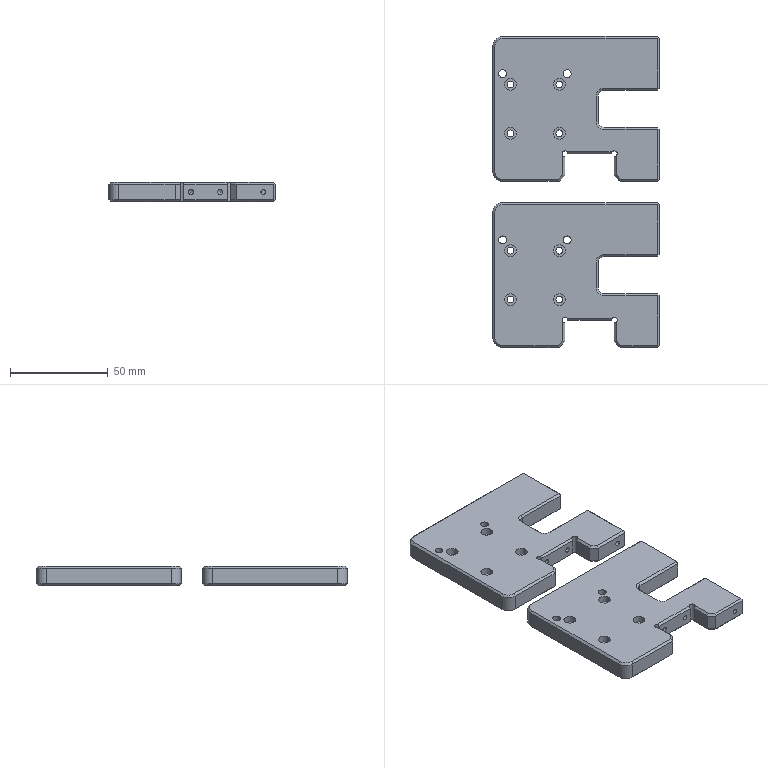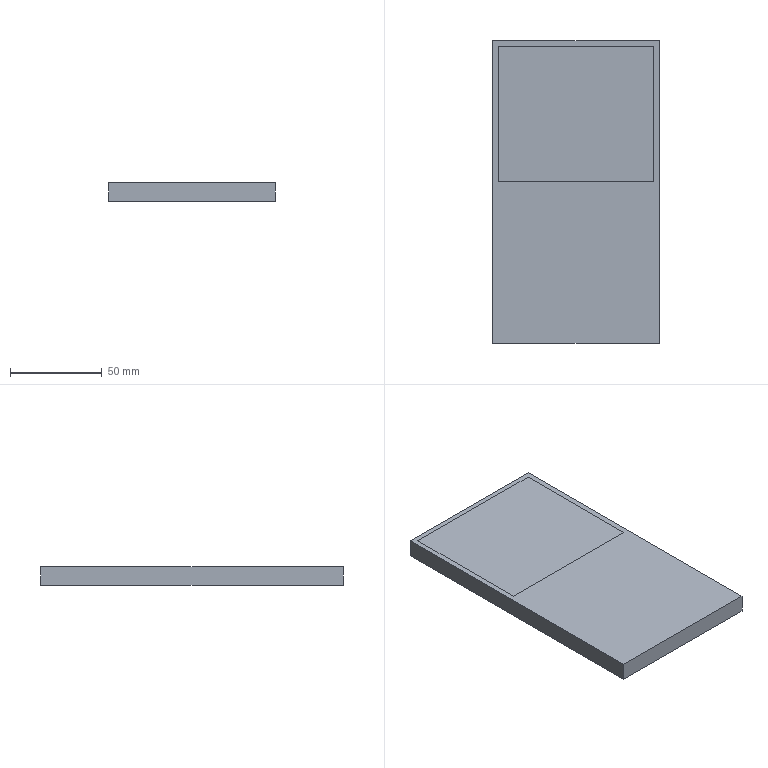CAM job | NX | 3+2 milling, drilling | part box 85 x 159 x 10 mm | stock box 91 x 165 x 10 mm
Tools:
number,name,description,diameter,corner_radius,flute_length,length,flutes
22,D6A45,Milling Tool-5 Parameters,6.0,0.0,3.0,3.0,2
20,D10,Milling Tool-5 Parameters,10.0,0.0,50.0,75.0,2
11,D10JING,Milling Tool-5 Parameters,10.0,0.0,50.0,75.0,2
19,3.0ZT,Drilling Tool,3.0,0.0,35.0,50.0,2
9,3.5ZT,Drilling Tool,3.5,0.0,35.0,50.0,2
15,D4,Milling Tool-5 Parameters,4.0,0.0,50.0,75.0,2
13,D3,Milling Tool-5 Parameters,3.0,0.0,50.0,75.0,2
Operations:
program,operation,operation_type,tool,method,geometry_group,spindle_rpm,surface_speed,feed_per_tooth,feed_cut,feed_plunge,cut_length_mm,path_length_mm,cut_time_min,machine_time_min
1AB胶-90-165-10毛胚,DRILLING_COPY_1_COPY_1,Operation,D6A45,METHOD,A,5000.0,94.0,0.025,250.0,0.0,60.0,528.786,0.24,0.2869
1AB胶-90-165-10毛胚,DRILLING_COPY_1_COPY_COPY_COPY_COPY_1_COPY_COPY_1,Operation,3.0ZT,METHOD,A,2000.0,20.0,0.0375,150.0,0.0,61.605,328.019,0.4107,0.4373
1AB胶-90-165-10毛胚,DRILLING_COPY_1_COPY_COPY_COPY_COPY_1_COPY_COPY_1_COPY_1,Operation,3.5ZT,METHOD,A,2000.0,20.0,0.0375,150.0,0.0,186.618,706.263,1.244,1.296
1AB胶-90-165-10毛胚,ZLEVEL_PROFILE_COPY,ZLevelMilling,D10,METHOD,A,7500.0,235.0,0.1667,2500.0,100.0,8636.868,8910.766,3.455,3.482
1AB胶-90-165-10毛胚,ZLEVEL_PROFILE_COPY_COPY_2,ZLevelMilling,D4,METHOD,A,7501.0,94.0,0.0933,1400.0,100.0,1528.521,3007.367,1.092,1.24
1AB胶-90-165-10毛胚,HOLE_MILLING_COPY,CylinderMilling,D4,METHOD,A,7500.0,141.0,0.0933,1400.0,100.0,579.071,1308.426,0.4136,0.4866
1AB胶-90-165-10毛胚,HOLE_MILLING_COPY_COPY,CylinderMilling,D3,METHOD,A,7500.0,70.0,0.0867,1300.0,100.0,544.536,979.717,0.4189,0.4624
1AB胶-90-165-10毛胚,ZLEVEL_PROFILE_1_COPY_1_COPY_COPY,ZLevelMilling,D6A45,METHOD,A,7500.0,141.0,0.0667,1000.0,100.0,962.646,2301.989,0.9626,1.097
1AB胶-90-165-10毛胚,刀补13,CylinderMilling,D3,METHOD,A,7500.0,70.0,0.0667,1000.0,100.0,142.865,578.046,0.1429,0.1864
1AB胶-90-165-10毛胚,刀补12,ZLevelMilling,D4,METHOD,A,3740.0,47.0,0.1337,1000.0,300.0,178.42,625.749,0.2824,0.3271
1AB胶-90-165-10毛胚,ZLEVEL_PROFILE_COPY_COPY_1,ZLevelMilling,D10JING,METHOD,A,7500.0,235.0,0.0667,1000.0,100.0,2607.791,2872.027,2.608,2.634
2,HOLE_MILLING_COPY_COPY_1,CylinderMilling,D4,METHOD,B,7500.0,141.0,0.08,1200.0,100.0,639.875,850.875,0.5332,0.5543
2,ZLEVEL_PROFILE_1_COPY_1_COPY_COPY_COPY,ZLevelMilling,D6A45,METHOD,B,7500.0,141.0,0.0667,1000.0,100.0,36.07,216.092,0.0361,0.0541
2,刀补13_COPY,CylinderMilling,D4,METHOD,B,7500.0,70.0,0.0667,1000.0,100.0,217.671,428.671,0.2177,0.2388